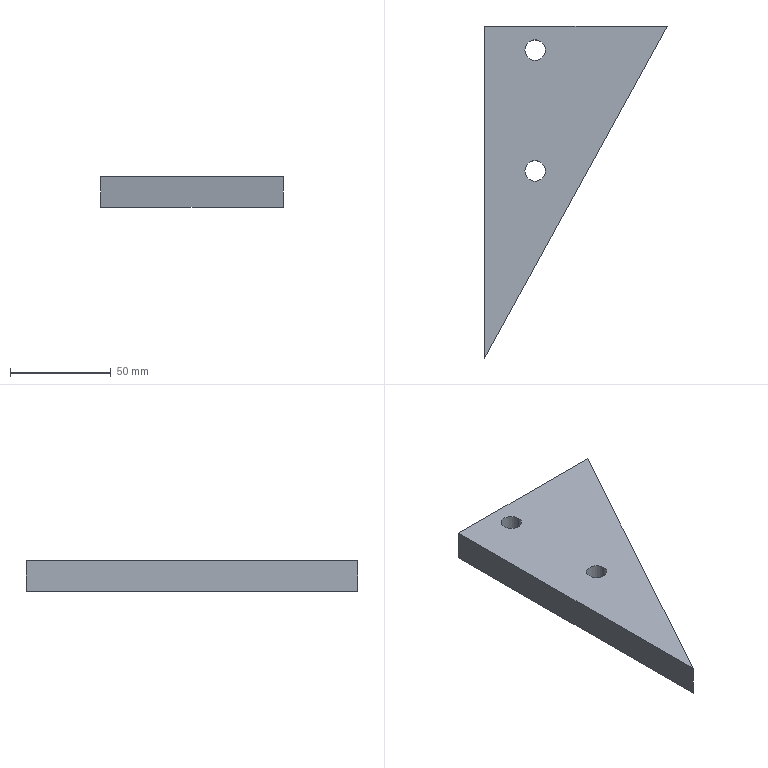Part | SolidWorks | features Extrusion 1, HoleWzd 1 | 1 solid | 9 faces | box 90.635 x 165 x 15 mm | volume 109709 mm3 | plane 5 | cylinder 4 | commonest cylinder face diameters 10.2 x4
STEP:
#1=CARTESIAN_POINT('',(-70.735,-12.,0.));
#2=VERTEX_POINT('',#1);
#3=CARTESIAN_POINT('',(-60.535,-12.,0.));
#4=VERTEX_POINT('',#3);
#5=CARTESIAN_POINT('',(-65.635,-12.,0.));
#6=DIRECTION('',(0.,0.,1.));
#7=DIRECTION('',(1.,0.,0.));
#8=AXIS2_PLACEMENT_3D('',#5,#6,#7);
#9=CIRCLE('',#8,5.1);
#10=EDGE_CURVE('',#2,#4,#9,.T.);
#11=ORIENTED_EDGE('',*,*,#10,.F.);
#12=CARTESIAN_POINT('',(-70.735,-12.,15.));
#13=VERTEX_POINT('',#12);
#14=CARTESIAN_POINT('',(-70.735,-12.,15.));
#15=DIRECTION('',(0.,0.,1.));
#16=VECTOR('',#15,1000.);
#17=LINE('',#14,#16);
#18=EDGE_CURVE('',#2,#13,#17,.T.);
#19=ORIENTED_EDGE('',*,*,#18,.T.);
#20=CARTESIAN_POINT('',(-60.535,-12.,15.));
#21=VERTEX_POINT('',#20);
#22=CARTESIAN_POINT('',(-65.635,-12.,15.));
#23=DIRECTION('',(0.,0.,1.));
#24=DIRECTION('',(1.,0.,0.));
#25=AXIS2_PLACEMENT_3D('',#22,#23,#24);
#26=CIRCLE('',#25,5.1);
#27=EDGE_CURVE('',#13,#21,#26,.T.);
#28=ORIENTED_EDGE('',*,*,#27,.T.);
#29=CARTESIAN_POINT('',(-60.535,-12.,15.));
#30=DIRECTION('',(0.,0.,1.));
#31=VECTOR('',#30,1000.);
#32=LINE('',#29,#31);
#33=EDGE_CURVE('',#4,#21,#32,.T.);
#34=ORIENTED_EDGE('',*,*,#33,.F.);
#35=EDGE_LOOP('',(#11,#19,#28,#34));
#36=FACE_OUTER_BOUND('',#35,.T.);
#37=CARTESIAN_POINT('',(-65.635,-12.,15.));
#38=DIRECTION('',(0.,0.,1.));
#39=DIRECTION('',(1.,0.,0.));
#40=AXIS2_PLACEMENT_3D('',#37,#38,#39);
#41=CYLINDRICAL_SURFACE('',#40,5.1);
#42=ADVANCED_FACE('',(#36),#41,.F.);
#43=CARTESIAN_POINT('',(-70.735,-72.,0.));
#44=VERTEX_POINT('',#43);
#45=CARTESIAN_POINT('',(-60.535,-72.,0.));
#46=VERTEX_POINT('',#45);
#47=CARTESIAN_POINT('',(-65.635,-72.,0.));
#48=DIRECTION('',(0.,0.,1.));
#49=DIRECTION('',(1.,0.,0.));
#50=AXIS2_PLACEMENT_3D('',#47,#48,#49);
#51=CIRCLE('',#50,5.1);
#52=EDGE_CURVE('',#44,#46,#51,.T.);
#53=ORIENTED_EDGE('',*,*,#52,.F.);
#54=CARTESIAN_POINT('',(-70.735,-72.,15.));
#55=VERTEX_POINT('',#54);
#56=CARTESIAN_POINT('',(-70.735,-72.,15.));
#57=DIRECTION('',(0.,0.,1.));
#58=VECTOR('',#57,1000.);
#59=LINE('',#56,#58);
#60=EDGE_CURVE('',#44,#55,#59,.T.);
#61=ORIENTED_EDGE('',*,*,#60,.T.);
#62=CARTESIAN_POINT('',(-60.535,-72.,15.));
#63=VERTEX_POINT('',#62);
#64=CARTESIAN_POINT('',(-65.635,-72.,15.));
#65=DIRECTION('',(0.,0.,1.));
#66=DIRECTION('',(1.,0.,0.));
#67=AXIS2_PLACEMENT_3D('',#64,#65,#66);
#68=CIRCLE('',#67,5.1);
#69=EDGE_CURVE('',#55,#63,#68,.T.);
#70=ORIENTED_EDGE('',*,*,#69,.T.);
#71=CARTESIAN_POINT('',(-60.535,-72.,15.));
#72=DIRECTION('',(0.,0.,1.));
#73=VECTOR('',#72,1000.);
#74=LINE('',#71,#73);
#75=EDGE_CURVE('',#46,#63,#74,.T.);
#76=ORIENTED_EDGE('',*,*,#75,.F.);
#77=EDGE_LOOP('',(#53,#61,#70,#76));
#78=FACE_OUTER_BOUND('',#77,.T.);
#79=CARTESIAN_POINT('',(-65.635,-72.,15.));
#80=DIRECTION('',(0.,0.,1.));
#81=DIRECTION('',(1.,0.,0.));
#82=AXIS2_PLACEMENT_3D('',#79,#80,#81);
#83=CYLINDRICAL_SURFACE('',#82,5.1);
#84=ADVANCED_FACE('',(#78),#83,.F.);
#85=CARTESIAN_POINT('',(-65.635,-12.,15.));
#86=DIRECTION('',(0.,0.,1.));
#87=DIRECTION('',(1.,0.,0.));
#88=AXIS2_PLACEMENT_3D('',#85,#86,#87);
#89=CIRCLE('',#88,5.1);
#90=EDGE_CURVE('',#21,#13,#89,.T.);
#91=ORIENTED_EDGE('',*,*,#90,.F.);
#92=ORIENTED_EDGE('',*,*,#27,.F.);
#93=EDGE_LOOP('',(#91,#92));
#94=FACE_BOUND('',#93,.T.);
#95=CARTESIAN_POINT('',(-65.635,-72.,15.));
#96=DIRECTION('',(0.,0.,1.));
#97=DIRECTION('',(1.,0.,0.));
#98=AXIS2_PLACEMENT_3D('',#95,#96,#97);
#99=CIRCLE('',#98,5.1);
#100=EDGE_CURVE('',#63,#55,#99,.T.);
#101=ORIENTED_EDGE('',*,*,#100,.F.);
#102=ORIENTED_EDGE('',*,*,#69,.F.);
#103=EDGE_LOOP('',(#101,#102));
#104=FACE_BOUND('',#103,.T.);
#105=CARTESIAN_POINT('',(-90.635,-165.,15.));
#106=VERTEX_POINT('',#105);
#107=CARTESIAN_POINT('',(0.,0.,15.));
#108=VERTEX_POINT('',#107);
#109=CARTESIAN_POINT('',(-90.635,-165.,15.));
#110=DIRECTION('',(0.4814,0.8765,0.));
#111=VECTOR('',#110,1000.);
#112=LINE('',#109,#111);
#113=EDGE_CURVE('',#106,#108,#112,.T.);
#114=ORIENTED_EDGE('',*,*,#113,.T.);
#115=CARTESIAN_POINT('',(-90.635,0.,15.));
#116=VERTEX_POINT('',#115);
#117=CARTESIAN_POINT('',(0.,0.,15.));
#118=DIRECTION('',(-1.,0.,0.));
#119=VECTOR('',#118,1000.);
#120=LINE('',#117,#119);
#121=EDGE_CURVE('',#108,#116,#120,.T.);
#122=ORIENTED_EDGE('',*,*,#121,.T.);
#123=CARTESIAN_POINT('',(-90.635,0.,15.));
#124=DIRECTION('',(0.,-1.,0.));
#125=VECTOR('',#124,1000.);
#126=LINE('',#123,#125);
#127=EDGE_CURVE('',#116,#106,#126,.T.);
#128=ORIENTED_EDGE('',*,*,#127,.T.);
#129=EDGE_LOOP('',(#114,#122,#128));
#130=FACE_OUTER_BOUND('',#129,.T.);
#131=CARTESIAN_POINT('',(0.,0.,15.));
#132=DIRECTION('',(0.,0.,1.));
#133=DIRECTION('',(1.,0.,0.));
#134=AXIS2_PLACEMENT_3D('',#131,#132,#133);
#135=PLANE('',#134);
#136=ADVANCED_FACE('',(#94,#104,#130),#135,.T.);
#137=CARTESIAN_POINT('',(-65.635,-12.,0.));
#138=DIRECTION('',(0.,0.,1.));
#139=DIRECTION('',(1.,0.,0.));
#140=AXIS2_PLACEMENT_3D('',#137,#138,#139);
#141=CIRCLE('',#140,5.1);
#142=EDGE_CURVE('',#4,#2,#141,.T.);
#143=ORIENTED_EDGE('',*,*,#142,.T.);
#144=ORIENTED_EDGE('',*,*,#10,.T.);
#145=EDGE_LOOP('',(#143,#144));
#146=FACE_BOUND('',#145,.T.);
#147=CARTESIAN_POINT('',(-65.635,-72.,0.));
#148=DIRECTION('',(0.,0.,1.));
#149=DIRECTION('',(1.,0.,0.));
#150=AXIS2_PLACEMENT_3D('',#147,#148,#149);
#151=CIRCLE('',#150,5.1);
#152=EDGE_CURVE('',#46,#44,#151,.T.);
#153=ORIENTED_EDGE('',*,*,#152,.T.);
#154=ORIENTED_EDGE('',*,*,#52,.T.);
#155=EDGE_LOOP('',(#153,#154));
#156=FACE_BOUND('',#155,.T.);
#157=CARTESIAN_POINT('',(-90.635,-165.,0.));
#158=VERTEX_POINT('',#157);
#159=CARTESIAN_POINT('',(0.,0.,0.));
#160=VERTEX_POINT('',#159);
#161=CARTESIAN_POINT('',(-90.635,-165.,0.));
#162=DIRECTION('',(0.4814,0.8765,0.));
#163=VECTOR('',#162,1000.);
#164=LINE('',#161,#163);
#165=EDGE_CURVE('',#158,#160,#164,.T.);
#166=ORIENTED_EDGE('',*,*,#165,.F.);
#167=CARTESIAN_POINT('',(-90.635,0.,0.));
#168=VERTEX_POINT('',#167);
#169=CARTESIAN_POINT('',(-90.635,0.,0.));
#170=DIRECTION('',(0.,-1.,0.));
#171=VECTOR('',#170,1000.);
#172=LINE('',#169,#171);
#173=EDGE_CURVE('',#168,#158,#172,.T.);
#174=ORIENTED_EDGE('',*,*,#173,.F.);
#175=CARTESIAN_POINT('',(0.,0.,0.));
#176=DIRECTION('',(-1.,0.,0.));
#177=VECTOR('',#176,1000.);
#178=LINE('',#175,#177);
#179=EDGE_CURVE('',#160,#168,#178,.T.);
#180=ORIENTED_EDGE('',*,*,#179,.F.);
#181=EDGE_LOOP('',(#166,#174,#180));
#182=FACE_OUTER_BOUND('',#181,.T.);
#183=CARTESIAN_POINT('',(0.,0.,0.));
#184=DIRECTION('',(0.,0.,1.));
#185=DIRECTION('',(1.,0.,0.));
#186=AXIS2_PLACEMENT_3D('',#183,#184,#185);
#187=PLANE('',#186);
#188=ADVANCED_FACE('',(#146,#156,#182),#187,.F.);
#189=ORIENTED_EDGE('',*,*,#165,.T.);
#190=CARTESIAN_POINT('',(0.,0.,15.));
#191=DIRECTION('',(0.,0.,-1.));
#192=VECTOR('',#191,1000.);
#193=LINE('',#190,#192);
#194=EDGE_CURVE('',#108,#160,#193,.T.);
#195=ORIENTED_EDGE('',*,*,#194,.F.);
#196=ORIENTED_EDGE('',*,*,#113,.F.);
#197=CARTESIAN_POINT('',(-90.635,-165.,15.));
#198=DIRECTION('',(0.,0.,-1.));
#199=VECTOR('',#198,1000.);
#200=LINE('',#197,#199);
#201=EDGE_CURVE('',#106,#158,#200,.T.);
#202=ORIENTED_EDGE('',*,*,#201,.T.);
#203=EDGE_LOOP('',(#189,#195,#196,#202));
#204=FACE_OUTER_BOUND('',#203,.T.);
#205=CARTESIAN_POINT('',(-90.635,-165.,15.));
#206=DIRECTION('',(-0.8765,0.4814,0.));
#207=DIRECTION('',(-0.4814,-0.8765,0.));
#208=AXIS2_PLACEMENT_3D('',#205,#206,#207);
#209=PLANE('',#208);
#210=ADVANCED_FACE('',(#204),#209,.F.);
#211=ORIENTED_EDGE('',*,*,#179,.T.);
#212=CARTESIAN_POINT('',(-90.635,0.,15.));
#213=DIRECTION('',(0.,0.,-1.));
#214=VECTOR('',#213,1000.);
#215=LINE('',#212,#214);
#216=EDGE_CURVE('',#116,#168,#215,.T.);
#217=ORIENTED_EDGE('',*,*,#216,.F.);
#218=ORIENTED_EDGE('',*,*,#121,.F.);
#219=ORIENTED_EDGE('',*,*,#194,.T.);
#220=EDGE_LOOP('',(#211,#217,#218,#219));
#221=FACE_OUTER_BOUND('',#220,.T.);
#222=CARTESIAN_POINT('',(0.,0.,15.));
#223=DIRECTION('',(0.,-1.,0.));
#224=DIRECTION('',(1.,0.,0.));
#225=AXIS2_PLACEMENT_3D('',#222,#223,#224);
#226=PLANE('',#225);
#227=ADVANCED_FACE('',(#221),#226,.F.);
#228=ORIENTED_EDGE('',*,*,#173,.T.);
#229=ORIENTED_EDGE('',*,*,#201,.F.);
#230=ORIENTED_EDGE('',*,*,#127,.F.);
#231=ORIENTED_EDGE('',*,*,#216,.T.);
#232=EDGE_LOOP('',(#228,#229,#230,#231));
#233=FACE_OUTER_BOUND('',#232,.T.);
#234=CARTESIAN_POINT('',(-90.635,0.,15.));
#235=DIRECTION('',(1.,0.,0.));
#236=DIRECTION('',(0.,0.,-1.));
#237=AXIS2_PLACEMENT_3D('',#234,#235,#236);
#238=PLANE('',#237);
#239=ADVANCED_FACE('',(#233),#238,.F.);
#240=ORIENTED_EDGE('',*,*,#60,.F.);
#241=ORIENTED_EDGE('',*,*,#152,.F.);
#242=ORIENTED_EDGE('',*,*,#75,.T.);
#243=ORIENTED_EDGE('',*,*,#100,.T.);
#244=EDGE_LOOP('',(#240,#241,#242,#243));
#245=FACE_OUTER_BOUND('',#244,.T.);
#246=CARTESIAN_POINT('',(-65.635,-72.,15.));
#247=DIRECTION('',(0.,0.,1.));
#248=DIRECTION('',(1.,0.,0.));
#249=AXIS2_PLACEMENT_3D('',#246,#247,#248);
#250=CYLINDRICAL_SURFACE('',#249,5.1);
#251=ADVANCED_FACE('',(#245),#250,.F.);
#252=ORIENTED_EDGE('',*,*,#18,.F.);
#253=ORIENTED_EDGE('',*,*,#142,.F.);
#254=ORIENTED_EDGE('',*,*,#33,.T.);
#255=ORIENTED_EDGE('',*,*,#90,.T.);
#256=EDGE_LOOP('',(#252,#253,#254,#255));
#257=FACE_OUTER_BOUND('',#256,.T.);
#258=CARTESIAN_POINT('',(-65.635,-12.,15.));
#259=DIRECTION('',(0.,0.,1.));
#260=DIRECTION('',(1.,0.,0.));
#261=AXIS2_PLACEMENT_3D('',#258,#259,#260);
#262=CYLINDRICAL_SURFACE('',#261,5.1);
#263=ADVANCED_FACE('',(#257),#262,.F.);
#264=CLOSED_SHELL('',(#42,#84,#136,#188,#210,#227,#239,#251,#263));
#265=MANIFOLD_SOLID_BREP('',#264);
#266=CARTESIAN_POINT('',(0.,0.,0.));
#267=DIRECTION('',(0.,0.,1.));
#268=DIRECTION('',(1.,0.,0.));
#269=AXIS2_PLACEMENT_3D('',#266,#267,#268);
#270=(LENGTH_UNIT()NAMED_UNIT(*)SI_UNIT(.MILLI.,.METRE.));
#271=UNCERTAINTY_MEASURE_WITH_UNIT(LENGTH_MEASURE(0.00001),#270,'','');
#272=(NAMED_UNIT(*)PLANE_ANGLE_UNIT()SI_UNIT($,.RADIAN.));
#273=(NAMED_UNIT(*)SI_UNIT($,.STERADIAN.)SOLID_ANGLE_UNIT());
#274=(GEOMETRIC_REPRESENTATION_CONTEXT(3)GLOBAL_UNCERTAINTY_ASSIGNED_CONTEXT((#271))GLOBAL_UNIT_ASSIGNED_CONTEXT((#270,#272,#273))REPRESENTATION_CONTEXT('',''));
#275=ADVANCED_BREP_SHAPE_REPRESENTATION('',(#265,#269),#274);